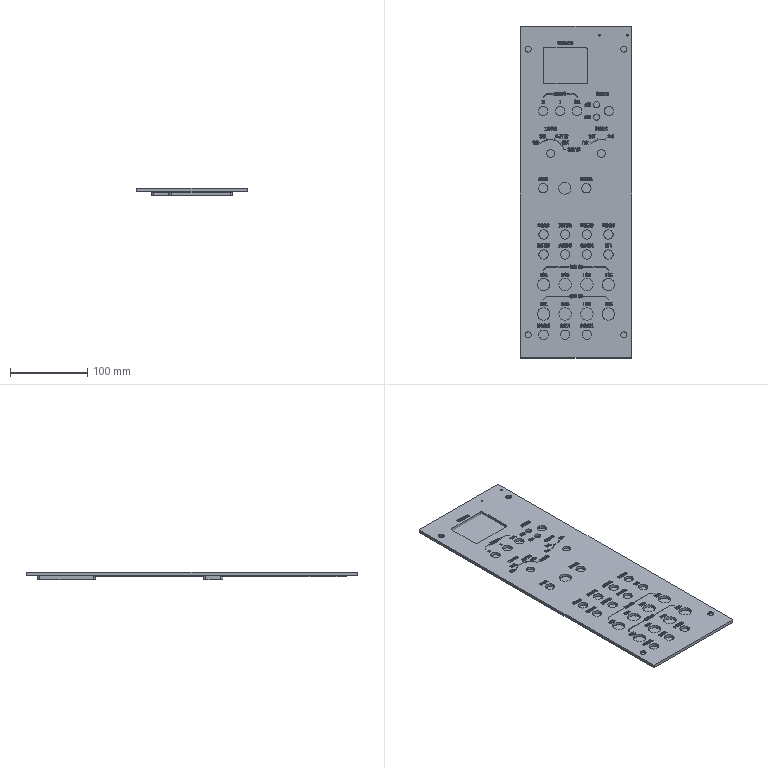Part | 1 solid | 6838 faces | volume 366894 mm3 | plane 4743 | other 1871 | cylinder 179 | spline 25 | cone 20 | commonest cylinder face diameters 6 x47 12.2 x32 2 x16 16.2 x16 2.5 x14 4 x14